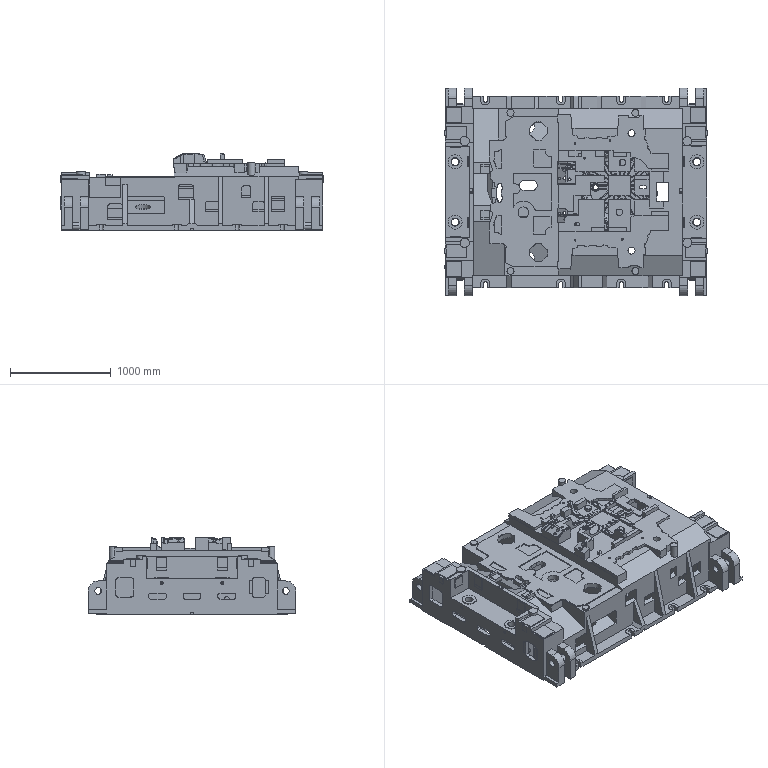Part | NX | features solid 2 | 1 solid | 1864 faces | box 2620 x 2060 x 758 mm | volume 857197509 mm3 | plane 1040 | spline 528 | cylinder 296 | commonest cylinder face diameters 100 x88 40 x78 50 x23 70 x17 90 x16 30 x13